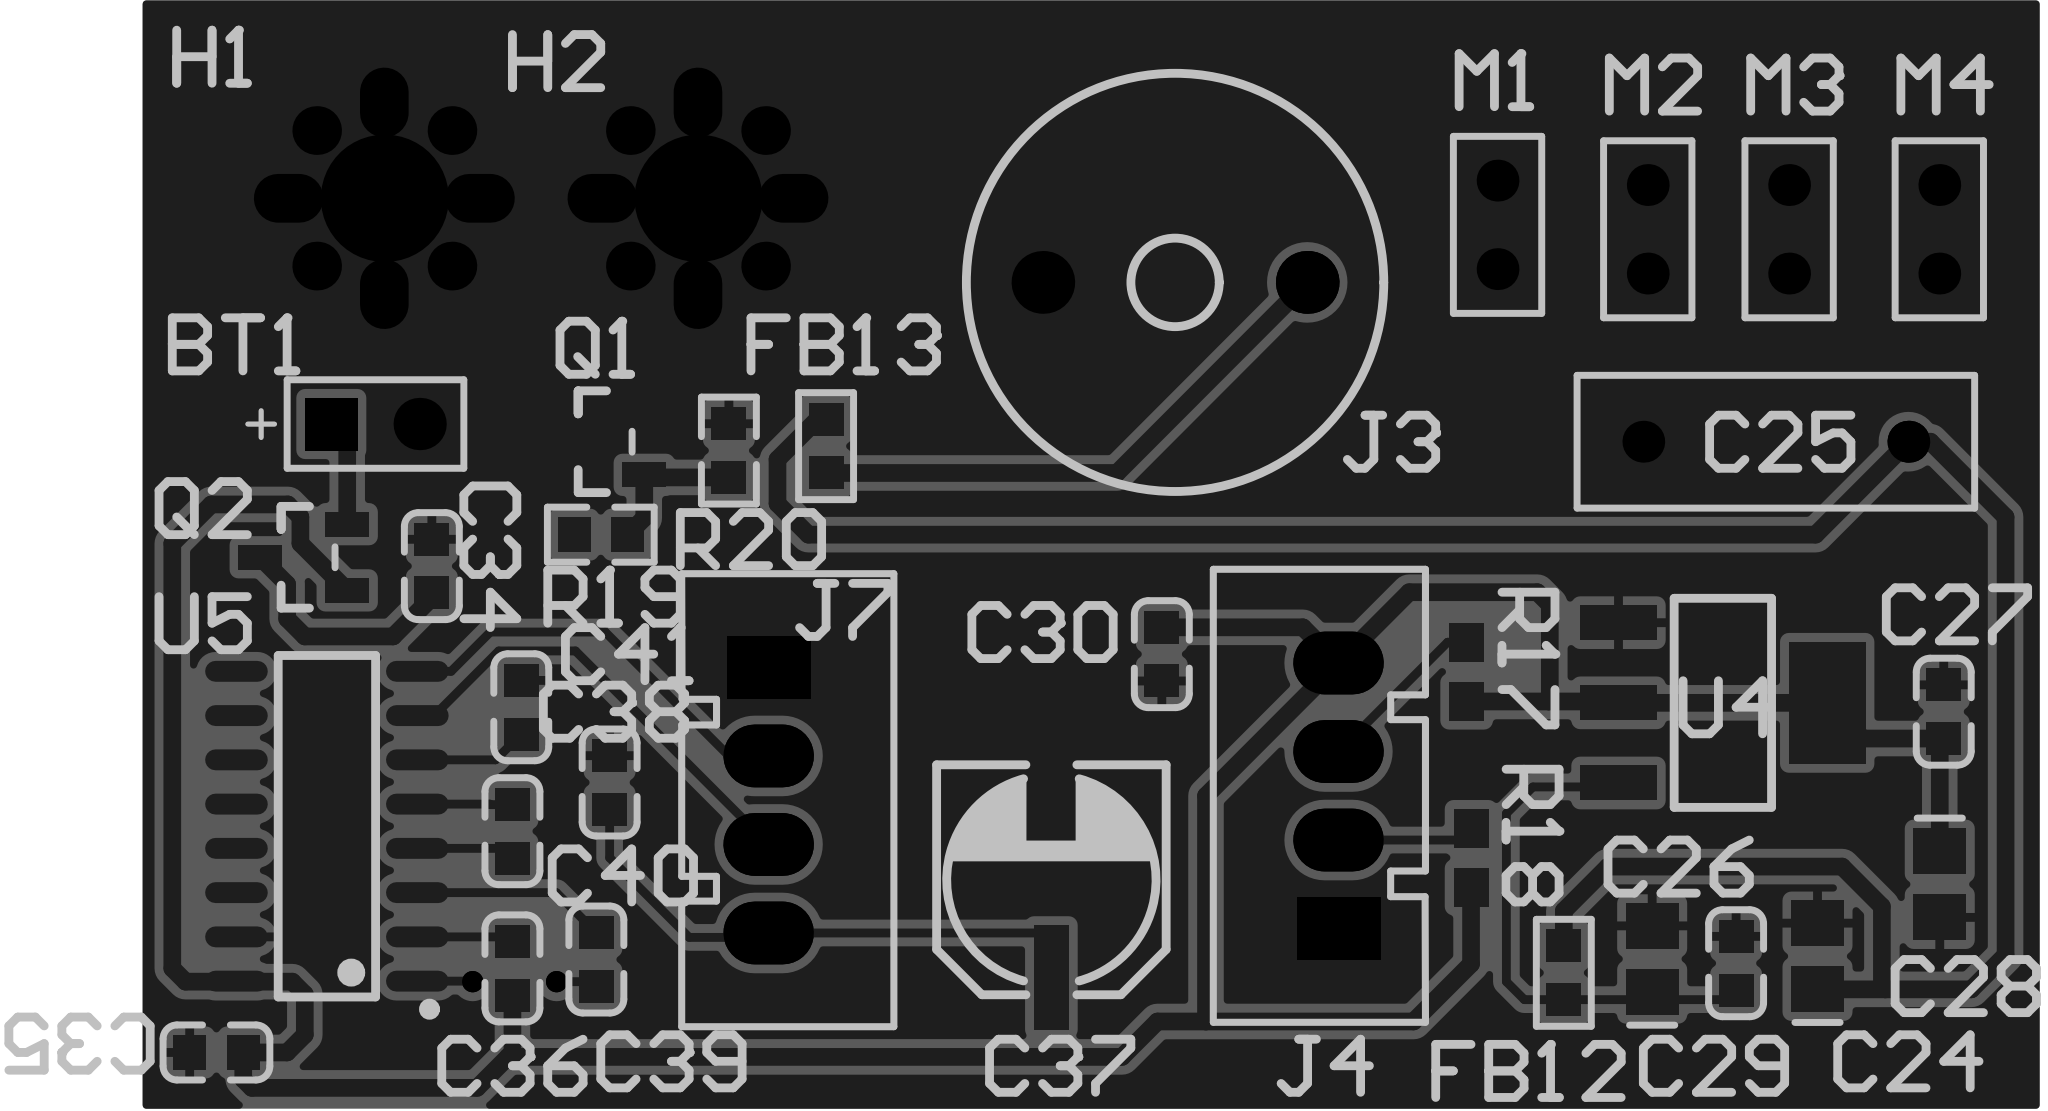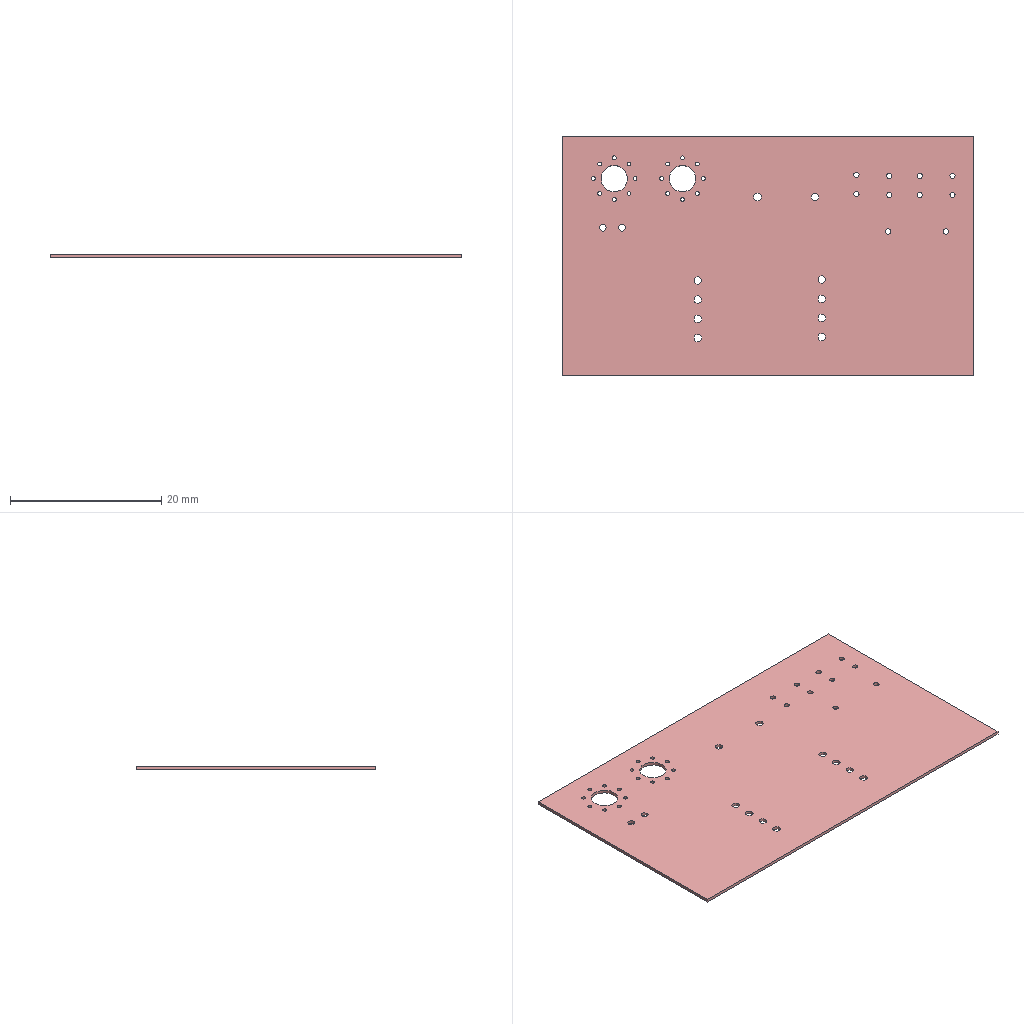Circuit board layout | Altium Designer | box 54.4 x 31.6 x 0.4 mm
Layer stack:
# Altium Designer layer stack of  (unit mm; dielectric type: 0 none, 1 core, 2 prepreg, 3 surface material)
index,name,kind,layer,copper_thickness_mm,dielectric_type,dielectric_thickness_mm,dielectric_material,dielectric_constant
0,Top Paste Mask Layer,other,,,,,,
1,Top Silkscreen Layer,other,,,,,,
2,Top Solder Mask Layer,dielectric,,,3,0.0102,Solder Resist,3.5
3,Top Layer,copper,Top Layer,0.0356,,,,
4,Dielectric1,dielectric,,,3,0.32,FR-4,4.8
5,Bottom Layer,copper,Bottom Layer,0.0356,,,,
6,Bottom Solder Mask Layer,dielectric,,,3,0.0102,Solder Resist,3.5
7,Bottom Silkscreen Layer,other,,,,,,
8,Bottom Paste Mask Layer,other,,,,,,
# drill layer pairs: low layer,high layer
drill_pair,Top Layer,Bottom Layer
Part placement:
Designator,Comment,Layer,Footprint,Center-X(mm),Center-Y(mm),Rotation
BT1,CR1200/NC,TopLayer,BAT-2,85.217,97.155,0
C24,,TopLayer,C0805,126.673,81.882,90
C25,,TopLayer,RAD-0.3,125.476,96.647,0
C26,,TopLayer,C0805,121.92,81.804,90
C27,Cap,TopLayer,0603_C,130.302,88.9,270
C28,,TopLayer,C0805,130.188,83.947,270
C29,Cap,TopLayer,0603_C,124.333,81.682,270
C30,Cap,TopLayer,0603_C,107.823,90.551,270
C34,Cap,TopLayer,0603_C,86.837,93.077,270
C35,Cap,TopLayer,0603_C,80.645,79.121,180
C36,Cap,TopLayer,0603_C,89.154,81.534,270
C37,Cap Pol1,TopLayer,CAP-SMD_BD6.3-L6.6-W6.6-FD,104.648,84.074,90
C38,Cap,TopLayer,0603_C,91.948,86.868,90
C39,Cap,TopLayer,0603_C,91.567,81.788,90
C40,Cap,TopLayer,0603_C,89.154,85.471,90
C41,Cap,TopLayer,0603_C,89.408,89.027,270
FB12,FB,TopLayer,0603_L,119.38,81.407,270
FB13,FB,TopLayer,0603_L,98.171,96.52,270
H1,H,TopLayer,HOLE-ZR,85.471,103.632,0
H2,H,TopLayer,HOLE-ZR,94.488,103.632,0
J3,BEEP,TopLayer,BUZ-TH_BD12.0-P7.60-D0.6-FD,108.204,101.219,180
J4,HEADER4X2.54MM,TopLayer,CN4$2F$DIP$2F$P2.54B,112.903,86.487,270
J7,HEADER4X2.54MM,TopLayer,CN4$2F$DIP$2F$P2.54B,96.52,86.36,90
M1,MARK,TopLayer,RAD-0.1,117.475,102.87,90
M2,MARK,TopLayer,RAD-0.1,121.793,102.743,90
M3,MARK,TopLayer,RAD-0.1,125.857,102.743,90
M4,MARK,TopLayer,RAD-0.1,130.175,102.743,90
Q1,S8050,TopLayer,SOT-23(SOT-23-3),91.694,96.647,0
Q2,BAT54C,TopLayer,SOT-23(SOT-23-3),83.154,93.331,0
R17,,TopLayer,J1-0603,116.586,90.043,270
R18,,TopLayer,J1-0603,116.713,84.709,270
R19,1K,TopLayer,0603_R,91.694,93.98,0
R20,10K,TopLayer,0603_R,95.377,96.393,270
U4,AMS1117-3.3V,TopLayer,SOT-223,123.952,89.154,180
U5,SP3232EEN,TopLayer,SOP-16_150MIL,83.82,85.613,90
Pad and via stacks:
# Altium Designer via and pad stacks of  (unit mm). Each distinct definition once, with the count of objects using it.
# via: kind,start_layer,end_layer,hole_mm,diameter_mm,mode(0 simple;1 top-mid-bottom;2 full stack),diameter_per_layer,count,example_net
# pad: kind,layer,hole_mm,hole_type(0 round;1 square;2 slot),plating,top_size,top_shape(1 round;2 rect;3 octagon;9 rounded rect),mid_size,bottom_size,mode,footprint,size_per_layer,count,example
pad,Multi-Layer,0.9,0,plated,1.5x1.5,2,1.5x1.5,1.5x1.5,0,BAT-2,,1,BT1.1
pad,Multi-Layer,0.9,0,plated,1.5x1.5,1,1.5x1.5,1.5x1.5,0,BAT-2,,1,BT1.2
pad,Multi-Layer,0.7,0,plated,1.2x1.2,1,1.2x1.2,1.2x1.2,0,RAD-0.3,,2,C25.1
pad,Multi-Layer,0.508,0,plated,1.397x1.397,1,1.397x1.397,1.397x1.397,0,HOLE-ZR,,8,H1.9
pad,Multi-Layer,0.508,0,plated,2x1.397,1,1.397x1.397,1.397x1.397,1,HOLE-ZR,,8,H1.8
pad,Multi-Layer,3.5,0,plated,3.65x3.65,1,3.65x3.65,3.65x3.65,0,HOLE-ZR,,2,H1.1
pad,Multi-Layer,1,0,plated,1.8x1.8,1,1.8x1.8,1.8x1.8,0,BUZ-TH_BD12.0-P7.60-D0.6-FD,,2,J3.2
pad,Multi-Layer,1,0,plated,2.6x1.8,1,2.6x1.8,2.6x1.8,0,CN4$2F$DIP$2F$P2.54B,,6,J4.4
pad,Multi-Layer,1,0,plated,2.4x1.8,2,2.4x1.8,2.4x1.8,0,CN4$2F$DIP$2F$P2.54B,,2,J4.1
pad,Multi-Layer,0.7,0,plated,1.2x1.2,1,1.2x1.2,1.2x1.2,0,RAD-0.1,,8,M1.2
pad,Top Layer,0,0,plated,1.5x1.3,2,1.5x1.3,1.5x1.3,0,C0805,,6,C24.1
pad,Top Layer,0,0,plated,0.98x0.93,2,0.98x0.93,0.98x0.93,0,0603_C,,20,C27.2
pad,Top Layer,0,0,plated,3x1,2,3x1,3x1,0,CAP-SMD_BD6.3-L6.6-W6.6-FD,,2,C37.2
pad,Top Layer,0,0,plated,0.98x0.93,2,0.98x0.93,0.98x0.93,0,0603_L,,4,FB12.1
pad,Top Layer,0,0,plated,1.25x0.7,2,1.25x0.7,1.25x0.7,0,SOT-23(SOT-23-3),,6,Q1.1
pad,Top Layer,0,0,plated,1x1.1,2,1x1.1,1x1.1,0,J1-0603,,4,R17.2
pad,Top Layer,0,0,plated,0.98x0.93,2,0.98x0.93,0.98x0.93,0,0603_R,,4,R19.1
pad,Top Layer,0,0,plated,2.2x1,2,2.2x1,2.2x1,0,SOT-223,,3,U4.1
pad,Top Layer,0,0,plated,3.5x2.2,2,3.5x2.2,3.5x2.2,0,SOT-223,,1,U4.4
pad,Top Layer,0,0,plated,1.8x0.6,1,1.8x0.6,1.8x0.6,0,SOP-16_150MIL,,16,U5.1
via,Top Layer,Bottom Layer,0.3048,0.6096,0,,2,$1N35
Copper pours:
name,layer,net,type(0 solid;1 hatched;2 none)
Top Layer-GND,Top Layer,GND,0
Bottom Layer-GND,Bottom Layer,GND,0
Design rules, without the lines most boards share:
# Altium Designer design rules of  (exported by Altium Designer, unit mm)
# columns: name | kind | enabled | priority | scope1 | scope2 | descriptor | typed fields (field=value)
Plane_PlaneConnect | 0 | disabled | 1 | All | All | Clearance Constraint (Gap=10mil) (Disabled)(All),(All) | gap=0.254
Plane_PlaneConnect_1 | 63 | disabled | 1 | All | All | Board Clearance Constraint (Gap=0mil) (Disabled)(All) |
Copper_PolygonConnect | 0 | disabled | 2 | All | All | Clearance Constraint (Gap=10mil) (Disabled)(All),(All) | gap=0.254
Copper_PolygonConnect_1 | 63 | disabled | 2 | All | All | Board Clearance Constraint (Gap=0mil) (Disabled)(All) |
Clearance | 0 | enabled | 3 | All | All | Clearance Constraint (Gap=10mil) (All),(All) | gap=0.254
Clearance_1 | 63 | enabled | 3 | All | All | Board Clearance Constraint (Gap=0mil) (All) |
otherClearance | 52 | enabled | 1 | All | All | Hole To Hole Clearance (Gap=11.8mil) (All),(All) | gap=0.2997
Width | 2 | enabled | 1 | All | All | Width Constraint (Min=10mil) (Max=90mil) (Preferred=10mil) (All) |
DiffPairsRouting | 51 | enabled | 1 | All | All | Differential Pairs Uncoupled Length using the Gap Constraints (Min=10mil) (Max=10mil) (Prefered=10mil)  and Width Constraints (Min=15mil) (Max=15mil) (Prefered=15mil) (All) |
RoutingVias | 11 | enabled | 1 | All | All | Routing Via (MinHoleWidth=28mil) (MaxHoleWidth=28mil) (PreferredHoleWidth=28mil) (MinWidth=50mil) (MaxWidth=50mil) (PreferedWidth=50mil) (All) | via_min_hole=0.7112 via_max_hole=0.7112 via_preferred_diameter=1.27 via_preferred_hole=0.7112
PlaneConnect | 6 | enabled | 1 | All | All | Power Plane Connect Rule(Relief Connect )(Expansion=20mil) (Conductor Width=10mil) (Air Gap=10mil) (Entries=4) (All) | relief_conductor_width=0.254 relief_entries=4 relief_expansion=0.508
PolygonConnect | 20 | enabled | 1 | All | All | Polygon Connect Rule(Relief Connect )(Conductor Width=10mil) (Relief Angle=90 Angle) (Entries=4) (Air Gap Width=10mil) (All),(All) | connect_style(0=relief,1=direct,2=none)=0 relief_conductor_width=0.254 relief_entries=4
PasteMaskExpansion | 14 | enabled | 1 | All | All | Paste Mask Expansion (Expansion =0mil) (All) | expansion=0
SolderMaskExpansion | 13 | enabled | 1 | All | All | Solder Mask Expansion (Expansion =4mil) (All) | expansion=0.1016